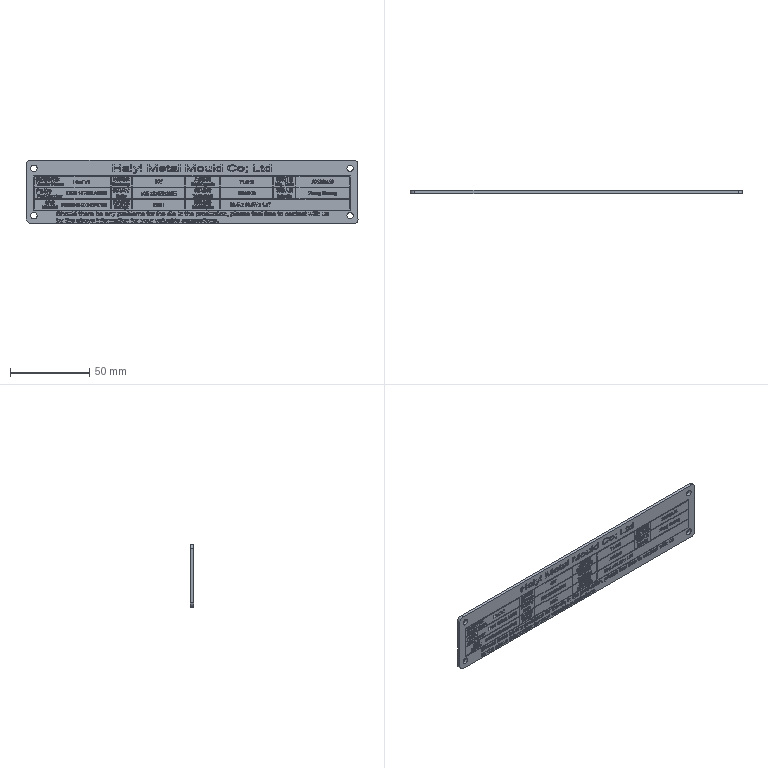Part | STEP file | gslz 2016.10.28-6_id1014_x_t | 1 solid | 9304 faces | volume 16189 mm3 | other 5312 | plane 3984 | cylinder 8 | commonest cylinder face diameters 4 x4 4.813 x2 6.245 x1 7.722 x1